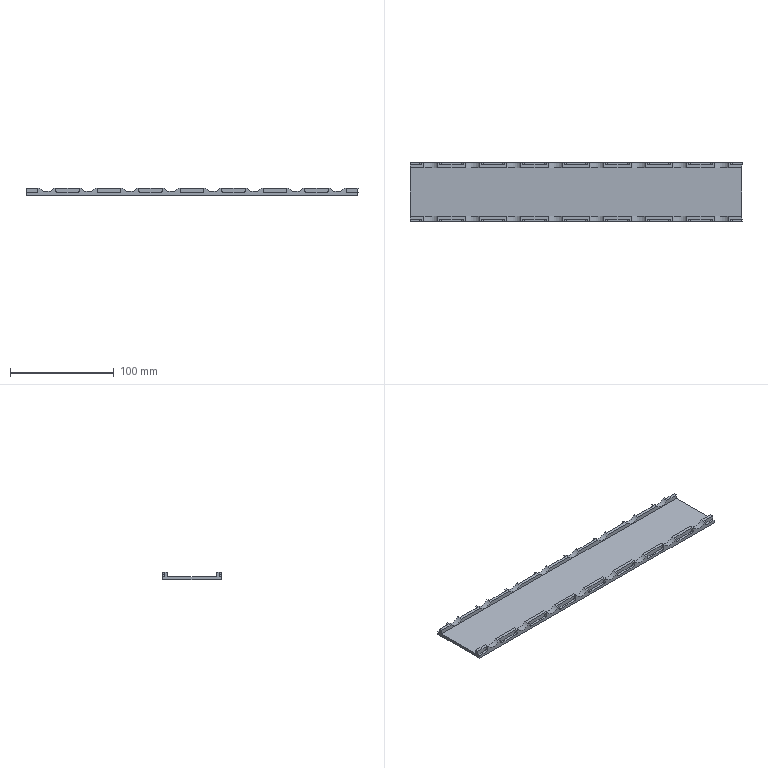NC program | Mastercam | posted with a generic post
Lines 1818 to 3883 of 9376, first 1896 of 2066 lines:
(8 FI |TOOL - 2|DIA. OFF. - 2|LEN. - 2|TOOL DIA. - 8.)
N3712 T2 M6
N3714 G0 G54 G90 X15.673 Y149.159 C0. B-90. S5000 M3
N3716 G43 H2 Z78.3
N3718 Z29.3
N3720 G1 Z22.3 F2000.
N3722 G41 D2 X9.609 Y143.942 F600.
N3724 G3 X7.8 Y140. I3.391 J-3.942
N3726 X9.609 Y136.058 I5.2
N3728 G1 G40 X15.673 Y130.841
N3730 G0 Z78.3
N3732 Y109.159
N3734 Z29.3
N3736 G1 Z22.3 F2000.
N3738 G41 D2 X9.609 Y103.942 F600.
N3740 G3 X7.8 Y100. I3.391 J-3.942
N3742 X9.609 Y96.058 I5.2
N3744 G1 G40 X15.673 Y90.841
N3746 G0 Z78.3
N3748 Y69.159
N3750 Z29.3
N3752 G1 Z22.3 F2000.
N3754 G41 D2 X9.609 Y63.942 F600.
N3756 G3 X7.8 Y60. I3.391 J-3.942
N3758 X9.609 Y56.058 I5.2
N3760 G1 G40 X15.673 Y50.841
N3762 G0 Z78.3
N3764 Y29.159
N3766 Z29.3
N3768 G1 Z22.3 F2000.
N3770 G41 D2 X9.609 Y23.942 F600.
N3772 G3 X7.8 Y20. I3.391 J-3.942
N3774 X9.609 Y16.058 I5.2
N3776 G1 G40 X15.673 Y10.841
N3778 G0 Z78.3
N3780 Y-10.841
N3782 Z29.3
N3784 G1 Z22.3 F2000.
N3786 G41 D2 X9.609 Y-16.058 F600.
N3788 G3 X7.8 Y-20. I3.391 J-3.942
N3790 X9.609 Y-23.942 I5.2
N3792 G1 G40 X15.673 Y-29.159
N3794 G0 Z78.3
N3796 Y-50.841
N3798 Z29.3
N3800 G1 Z22.3 F2000.
N3802 G41 D2 X9.609 Y-56.058 F600.
N3804 G3 X7.8 Y-60. I3.391 J-3.942
N3806 X9.609 Y-63.942 I5.2
N3808 G1 G40 X15.673 Y-69.159
N3810 G0 Z78.3
N3812 Y-90.841
N3814 Z29.3
N3816 G1 Z22.3 F2000.
N3818 G41 D2 X9.609 Y-96.058 F600.
N3820 G3 X7.8 Y-100. I3.391 J-3.942
N3822 X9.609 Y-103.942 I5.2
N3824 G1 G40 X15.673 Y-109.159
N3826 G0 Z78.3
N3828 Y-130.841
N3830 Z29.3
N3832 G1 Z22.3 F2000.
N3834 G41 D2 X9.609 Y-136.058 F600.
N3836 G3 X7.8 Y-140. I3.391 J-3.942
N3838 X9.609 Y-143.942 I5.2
N3840 G1 G40 X15.673 Y-149.159
N3842 G0 Z78.3
N3844 M5
N3846 G0 G28 G91 Z0.
N3848 G28 B0.
N3850 M01
N3852 G0 G17 G40 G80 G90 G94 G98
N3854 G0 G28 G91 Z0.
(4 RC |TOOL - 3|DIA. OFF. - 3|LEN. - 3|TOOL DIA. - 4.)
N3856 T3 M6
N3858 G0 G54 G90 X5.1 Y164. C0. B-90. S6500 M3
N3860 G43 H3 Z78.3
N3862 Z32.3
N3864 G1 Z31. F2000.
N3866 G41 D3 Y160. F600.
N3868 Y150.6
N3870 X7.
N3872 G40 X11.
N3874 Z30.7 F2000.
N3876 G42 D3 X7. F600.
N3878 X5.1
N3880 Y160.
N3882 G40 Y164.
N3884 Z30.4 F2000.
N3886 G41 D3 Y160. F600.
N3888 Y150.6
N3890 X7.
N3892 G40 X11.
N3894 Z30.1 F2000.
N3896 G42 D3 X7. F600.
N3898 X5.1
N3900 Y160.
N3902 G40 Y164.
N3904 Z29.8 F2000.
N3906 G41 D3 Y160. F600.
N3908 Y150.6
N3910 X7.
N3912 G40 X11.
N3914 Z29.5 F2000.
N3916 G42 D3 X7. F600.
N3918 X5.1
N3920 Y160.
N3922 G40 Y164.
N3924 Z29.2 F2000.
N3926 G41 D3 Y160. F600.
N3928 Y150.6
N3930 X7.
N3932 G40 X11.
N3934 Z28.9 F2000.
N3936 G42 D3 X7. F600.
N3938 X5.1
N3940 Y160.
N3942 G40 Y164.
N3944 Z28.6 F2000.
N3946 G41 D3 Y160. F600.
N3948 Y150.6
N3950 X7.
N3952 G40 X11.
N3954 Z28.3 F2000.
N3956 G42 D3 X7. F600.
N3958 X5.1
N3960 Y160.
N3962 G40 Y164.
N3964 Z28. F2000.
N3966 G41 D3 Y160. F600.
N3968 Y150.6
N3970 X7.
N3972 G40 X11.
N3974 Z27.7 F2000.
N3976 G42 D3 X7. F600.
N3978 X5.1
N3980 Y160.
N3982 G40 Y164.
N3984 Z27.4 F2000.
N3986 G41 D3 Y160. F600.
N3988 Y150.6
N3990 X7.
N3992 G40 X11.
N3994 Z27.1 F2000.
N3996 G42 D3 X7. F600.
N3998 X5.1
N4000 Y160.
N4002 G40 Y164.
N4004 Z26.8 F2000.
N4006 G41 D3 Y160. F600.
N4008 Y150.6
N4010 X7.
N4012 G40 X11.
N4014 Z26.5 F2000.
N4016 G42 D3 X7. F600.
N4018 X5.1
N4020 Y160.
N4022 G40 Y164.
N4024 Z26.2 F2000.
N4026 G41 D3 Y160. F600.
N4028 Y150.6
N4030 X7.
N4032 G40 X11.
N4034 G0 Z78.3
N4036 Y129.4
N4038 Z32.3
N4040 G1 Z31. F2000.
N4042 G41 D3 X7. F600.
N4044 X5.1
N4046 Y110.6
N4048 X7.
N4050 G40 X11.
N4052 Z30.7 F2000.
N4054 G42 D3 X7. F600.
N4056 X5.1
N4058 Y129.4
N4060 X7.
N4062 G40 X11.
N4064 Z30.4 F2000.
N4066 G41 D3 X7. F600.
N4068 X5.1
N4070 Y110.6
N4072 X7.
N4074 G40 X11.
N4076 Z30.1 F2000.
N4078 G42 D3 X7. F600.
N4080 X5.1
N4082 Y129.4
N4084 X7.
N4086 G40 X11.
N4088 Z29.8 F2000.
N4090 G41 D3 X7. F600.
N4092 X5.1
N4094 Y110.6
N4096 X7.
N4098 G40 X11.
N4100 Z29.5 F2000.
N4102 G42 D3 X7. F600.
N4104 X5.1
N4106 Y129.4
N4108 X7.
N4110 G40 X11.
N4112 Z29.2 F2000.
N4114 G41 D3 X7. F600.
N4116 X5.1
N4118 Y110.6
N4120 X7.
N4122 G40 X11.
N4124 Z28.9 F2000.
N4126 G42 D3 X7. F600.
N4128 X5.1
N4130 Y129.4
N4132 X7.
N4134 G40 X11.
N4136 Z28.6 F2000.
N4138 G41 D3 X7. F600.
N4140 X5.1
N4142 Y110.6
N4144 X7.
N4146 G40 X11.
N4148 Z28.3 F2000.
N4150 G42 D3 X7. F600.
N4152 X5.1
N4154 Y129.4
N4156 X7.
N4158 G40 X11.
N4160 Z28. F2000.
N4162 G41 D3 X7. F600.
N4164 X5.1
N4166 Y110.6
N4168 X7.
N4170 G40 X11.
N4172 Z27.7 F2000.
N4174 G42 D3 X7. F600.
N4176 X5.1
N4178 Y129.4
N4180 X7.
N4182 G40 X11.
N4184 Z27.4 F2000.
N4186 G41 D3 X7. F600.
N4188 X5.1
N4190 Y110.6
N4192 X7.
N4194 G40 X11.
N4196 Z27.1 F2000.
N4198 G42 D3 X7. F600.
N4200 X5.1
N4202 Y129.4
N4204 X7.
N4206 G40 X11.
N4208 Z26.8 F2000.
N4210 G41 D3 X7. F600.
N4212 X5.1
N4214 Y110.6
N4216 X7.
N4218 G40 X11.
N4220 Z26.5 F2000.
N4222 G42 D3 X7. F600.
N4224 X5.1
N4226 Y129.4
N4228 X7.
N4230 G40 X11.
N4232 Z26.2 F2000.
N4234 G41 D3 X7. F600.
N4236 X5.1
N4238 Y110.6
N4240 X7.
N4242 G40 X11.
N4244 G0 Z78.3
N4246 Y89.4
N4248 Z32.3
N4250 G1 Z31. F2000.
N4252 G41 D3 X7. F600.
N4254 X5.1
N4256 Y70.6
N4258 X7.
N4260 G40 X11.
N4262 Z30.7 F2000.
N4264 G42 D3 X7. F600.
N4266 X5.1
N4268 Y89.4
N4270 X7.
N4272 G40 X11.
N4274 Z30.4 F2000.
N4276 G41 D3 X7. F600.
N4278 X5.1
N4280 Y70.6
N4282 X7.
N4284 G40 X11.
N4286 Z30.1 F2000.
N4288 G42 D3 X7. F600.
N4290 X5.1
N4292 Y89.4
N4294 X7.
N4296 G40 X11.
N4298 Z29.8 F2000.
N4300 G41 D3 X7. F600.
N4302 X5.1
N4304 Y70.6
N4306 X7.
N4308 G40 X11.
N4310 Z29.5 F2000.
N4312 G42 D3 X7. F600.
N4314 X5.1
N4316 Y89.4
N4318 X7.
N4320 G40 X11.
N4322 Z29.2 F2000.
N4324 G41 D3 X7. F600.
N4326 X5.1
N4328 Y70.6
N4330 X7.
N4332 G40 X11.
N4334 Z28.9 F2000.
N4336 G42 D3 X7. F600.
N4338 X5.1
N4340 Y89.4
N4342 X7.
N4344 G40 X11.
N4346 Z28.6 F2000.
N4348 G41 D3 X7. F600.
N4350 X5.1
N4352 Y70.6
N4354 X7.
N4356 G40 X11.
N4358 Z28.3 F2000.
N4360 G42 D3 X7. F600.
N4362 X5.1
N4364 Y89.4
N4366 X7.
N4368 G40 X11.
N4370 Z28. F2000.
N4372 G41 D3 X7. F600.
N4374 X5.1
N4376 Y70.6
N4378 X7.
N4380 G40 X11.
N4382 Z27.7 F2000.
N4384 G42 D3 X7. F600.
N4386 X5.1
N4388 Y89.4
N4390 X7.
N4392 G40 X11.
N4394 Z27.4 F2000.
N4396 G41 D3 X7. F600.
N4398 X5.1
N4400 Y70.6
N4402 X7.
N4404 G40 X11.
N4406 Z27.1 F2000.
N4408 G42 D3 X7. F600.
N4410 X5.1
N4412 Y89.4
N4414 X7.
N4416 G40 X11.
N4418 Z26.8 F2000.
N4420 G41 D3 X7. F600.
N4422 X5.1
N4424 Y70.6
N4426 X7.
N4428 G40 X11.
N4430 Z26.5 F2000.
N4432 G42 D3 X7. F600.
N4434 X5.1
N4436 Y89.4
N4438 X7.
N4440 G40 X11.
N4442 Z26.2 F2000.
N4444 G41 D3 X7. F600.
N4446 X5.1
N4448 Y70.6
N4450 X7.
N4452 G40 X11.
N4454 G0 Z78.3
N4456 Y49.4
N4458 Z32.3
N4460 G1 Z31. F2000.
N4462 G41 D3 X7. F600.
N4464 X5.1
N4466 Y30.6
N4468 X7.
N4470 G40 X11.
N4472 Z30.7 F2000.
N4474 G42 D3 X7. F600.
N4476 X5.1
N4478 Y49.4
N4480 X7.
N4482 G40 X11.
N4484 Z30.4 F2000.
N4486 G41 D3 X7. F600.
N4488 X5.1
N4490 Y30.6
N4492 X7.
N4494 G40 X11.
N4496 Z30.1 F2000.
N4498 G42 D3 X7. F600.
N4500 X5.1
N4502 Y49.4
N4504 X7.
N4506 G40 X11.
N4508 Z29.8 F2000.
N4510 G41 D3 X7. F600.
N4512 X5.1
N4514 Y30.6
N4516 X7.
N4518 G40 X11.
N4520 Z29.5 F2000.
N4522 G42 D3 X7. F600.
N4524 X5.1
N4526 Y49.4
N4528 X7.
N4530 G40 X11.
N4532 Z29.2 F2000.
N4534 G41 D3 X7. F600.
N4536 X5.1
N4538 Y30.6
N4540 X7.
N4542 G40 X11.
N4544 Z28.9 F2000.
N4546 G42 D3 X7. F600.
N4548 X5.1
N4550 Y49.4
N4552 X7.
N4554 G40 X11.
N4556 Z28.6 F2000.
N4558 G41 D3 X7. F600.
N4560 X5.1
N4562 Y30.6
N4564 X7.
N4566 G40 X11.
N4568 Z28.3 F2000.
N4570 G42 D3 X7. F600.
N4572 X5.1
N4574 Y49.4
N4576 X7.
N4578 G40 X11.
N4580 Z28. F2000.
N4582 G41 D3 X7. F600.
N4584 X5.1
N4586 Y30.6
N4588 X7.
N4590 G40 X11.
N4592 Z27.7 F2000.
N4594 G42 D3 X7. F600.
N4596 X5.1
N4598 Y49.4
N4600 X7.
N4602 G40 X11.
N4604 Z27.4 F2000.
N4606 G41 D3 X7. F600.
N4608 X5.1
N4610 Y30.6
N4612 X7.
N4614 G40 X11.
N4616 Z27.1 F2000.
N4618 G42 D3 X7. F600.
N4620 X5.1
N4622 Y49.4
N4624 X7.
N4626 G40 X11.
N4628 Z26.8 F2000.
N4630 G41 D3 X7. F600.
N4632 X5.1
N4634 Y30.6
N4636 X7.
N4638 G40 X11.
N4640 Z26.5 F2000.
N4642 G42 D3 X7. F600.
N4644 X5.1
N4646 Y49.4
N4648 X7.
N4650 G40 X11.
N4652 Z26.2 F2000.
N4654 G41 D3 X7. F600.
N4656 X5.1
N4658 Y30.6
N4660 X7.
N4662 G40 X11.
N4664 G0 Z78.3
N4666 Y9.4
N4668 Z32.3
N4670 G1 Z31. F2000.
N4672 G41 D3 X7. F600.
N4674 X5.1
N4676 Y-9.4
N4678 X7.
N4680 G40 X11.
N4682 Z30.7 F2000.
N4684 G42 D3 X7. F600.
N4686 X5.1
N4688 Y9.4
N4690 X7.
N4692 G40 X11.
N4694 Z30.4 F2000.
N4696 G41 D3 X7. F600.
N4698 X5.1
N4700 Y-9.4
N4702 X7.
N4704 G40 X11.
N4706 Z30.1 F2000.
N4708 G42 D3 X7. F600.
N4710 X5.1
N4712 Y9.4
N4714 X7.
N4716 G40 X11.
N4718 Z29.8 F2000.
N4720 G41 D3 X7. F600.
N4722 X5.1
N4724 Y-9.4
N4726 X7.
N4728 G40 X11.
N4730 Z29.5 F2000.
N4732 G42 D3 X7. F600.
N4734 X5.1
N4736 Y9.4
N4738 X7.
N4740 G40 X11.
N4742 Z29.2 F2000.
N4744 G41 D3 X7. F600.
N4746 X5.1
N4748 Y-9.4
N4750 X7.
N4752 G40 X11.
N4754 Z28.9 F2000.
N4756 G42 D3 X7. F600.
N4758 X5.1
N4760 Y9.4
N4762 X7.
N4764 G40 X11.
N4766 Z28.6 F2000.
N4768 G41 D3 X7. F600.
N4770 X5.1
N4772 Y-9.4
N4774 X7.
N4776 G40 X11.
N4778 Z28.3 F2000.
N4780 G42 D3 X7. F600.
N4782 X5.1
N4784 Y9.4
N4786 X7.
N4788 G40 X11.
N4790 Z28. F2000.
N4792 G41 D3 X7. F600.
N4794 X5.1
N4796 Y-9.4
N4798 X7.
N4800 G40 X11.
N4802 Z27.7 F2000.
N4804 G42 D3 X7. F600.
N4806 X5.1
N4808 Y9.4
N4810 X7.
N4812 G40 X11.
N4814 Z27.4 F2000.
N4816 G41 D3 X7. F600.
N4818 X5.1
N4820 Y-9.4
N4822 X7.
N4824 G40 X11.
N4826 Z27.1 F2000.
N4828 G42 D3 X7. F600.
N4830 X5.1
N4832 Y9.4
N4834 X7.
N4836 G40 X11.
N4838 Z26.8 F2000.
N4840 G41 D3 X7. F600.
N4842 X5.1
N4844 Y-9.4
N4846 X7.
N4848 G40 X11.
N4850 Z26.5 F2000.
N4852 G42 D3 X7. F600.
N4854 X5.1
N4856 Y9.4
N4858 X7.
N4860 G40 X11.
N4862 Z26.2 F2000.
N4864 G41 D3 X7. F600.
N4866 X5.1
N4868 Y-9.4
N4870 X7.
N4872 G40 X11.
N4874 G0 Z78.3
N4876 Y-30.6
N4878 Z32.3
N4880 G1 Z31. F2000.
N4882 G41 D3 X7. F600.
N4884 X5.1
N4886 Y-49.4
N4888 X7.
N4890 G40 X11.
N4892 Z30.7 F2000.
N4894 G42 D3 X7. F600.
N4896 X5.1
N4898 Y-30.6
N4900 X7.
N4902 G40 X11.
N4904 Z30.4 F2000.
N4906 G41 D3 X7. F600.
N4908 X5.1
N4910 Y-49.4
N4912 X7.
N4914 G40 X11.
N4916 Z30.1 F2000.
N4918 G42 D3 X7. F600.
N4920 X5.1
N4922 Y-30.6
N4924 X7.
N4926 G40 X11.
N4928 Z29.8 F2000.
N4930 G41 D3 X7. F600.
N4932 X5.1
N4934 Y-49.4
N4936 X7.
N4938 G40 X11.
N4940 Z29.5 F2000.
N4942 G42 D3 X7. F600.
N4944 X5.1
N4946 Y-30.6
N4948 X7.
N4950 G40 X11.
N4952 Z29.2 F2000.
N4954 G41 D3 X7. F600.
N4956 X5.1
N4958 Y-49.4
N4960 X7.
N4962 G40 X11.
N4964 Z28.9 F2000.
N4966 G42 D3 X7. F600.
N4968 X5.1
N4970 Y-30.6
N4972 X7.
N4974 G40 X11.
N4976 Z28.6 F2000.
N4978 G41 D3 X7. F600.
N4980 X5.1
N4982 Y-49.4
N4984 X7.
N4986 G40 X11.
N4988 Z28.3 F2000.
N4990 G42 D3 X7. F600.
N4992 X5.1
N4994 Y-30.6
N4996 X7.
N4998 G40 X11.
N5000 Z28. F2000.
N5002 G41 D3 X7. F600.
N5004 X5.1
N5006 Y-49.4
N5008 X7.
N5010 G40 X11.
N5012 Z27.7 F2000.
N5014 G42 D3 X7. F600.
N5016 X5.1
N5018 Y-30.6
N5020 X7.
N5022 G40 X11.
N5024 Z27.4 F2000.
N5026 G41 D3 X7. F600.
N5028 X5.1
N5030 Y-49.4
N5032 X7.
N5034 G40 X11.
N5036 Z27.1 F2000.
N5038 G42 D3 X7. F600.
N5040 X5.1
N5042 Y-30.6
N5044 X7.
N5046 G40 X11.
N5048 Z26.8 F2000.
N5050 G41 D3 X7. F600.
N5052 X5.1
N5054 Y-49.4
N5056 X7.
N5058 G40 X11.
N5060 Z26.5 F2000.
N5062 G42 D3 X7. F600.
N5064 X5.1
N5066 Y-30.6
N5068 X7.
N5070 G40 X11.
N5072 Z26.2 F2000.
N5074 G41 D3 X7. F600.
N5076 X5.1
N5078 Y-49.4
N5080 X7.
N5082 G40 X11.
N5084 G0 Z78.3
N5086 Y-70.6
N5088 Z32.3
N5090 G1 Z31. F2000.
N5092 G41 D3 X7. F600.
N5094 X5.1
N5096 Y-89.4
N5098 X7.
N5100 G40 X11.
N5102 Z30.7 F2000.
N5104 G42 D3 X7. F600.
N5106 X5.1
N5108 Y-70.6
N5110 X7.
N5112 G40 X11.
N5114 Z30.4 F2000.
N5116 G41 D3 X7. F600.
N5118 X5.1
N5120 Y-89.4
N5122 X7.
N5124 G40 X11.
N5126 Z30.1 F2000.
N5128 G42 D3 X7. F600.
N5130 X5.1
N5132 Y-70.6
N5134 X7.
N5136 G40 X11.
N5138 Z29.8 F2000.
N5140 G41 D3 X7. F600.
N5142 X5.1
N5144 Y-89.4
N5146 X7.
N5148 G40 X11.
N5150 Z29.5 F2000.
N5152 G42 D3 X7. F600.
N5154 X5.1
N5156 Y-70.6
N5158 X7.
N5160 G40 X11.
N5162 Z29.2 F2000.
N5164 G41 D3 X7. F600.
N5166 X5.1
N5168 Y-89.4
N5170 X7.
N5172 G40 X11.
N5174 Z28.9 F2000.
N5176 G42 D3 X7. F600.
N5178 X5.1
N5180 Y-70.6
N5182 X7.
N5184 G40 X11.
N5186 Z28.6 F2000.
N5188 G41 D3 X7. F600.
N5190 X5.1
N5192 Y-89.4
N5194 X7.
N5196 G40 X11.
N5198 Z28.3 F2000.
N5200 G42 D3 X7. F600.
N5202 X5.1
N5204 Y-70.6
N5206 X7.
N5208 G40 X11.
N5210 Z28. F2000.
N5212 G41 D3 X7. F600.
N5214 X5.1
N5216 Y-89.4
N5218 X7.
N5220 G40 X11.
N5222 Z27.7 F2000.
N5224 G42 D3 X7. F600.
N5226 X5.1
N5228 Y-70.6
N5230 X7.
N5232 G40 X11.
N5234 Z27.4 F2000.
N5236 G41 D3 X7. F600.
N5238 X5.1
N5240 Y-89.4
N5242 X7.
N5244 G40 X11.
N5246 Z27.1 F2000.
N5248 G42 D3 X7. F600.
N5250 X5.1
N5252 Y-70.6
N5254 X7.
N5256 G40 X11.
N5258 Z26.8 F2000.
N5260 G41 D3 X7. F600.
N5262 X5.1
N5264 Y-89.4
N5266 X7.
N5268 G40 X11.
N5270 Z26.5 F2000.
N5272 G42 D3 X7. F600.
N5274 X5.1
N5276 Y-70.6
N5278 X7.
N5280 G40 X11.
N5282 Z26.2 F2000.
N5284 G41 D3 X7. F600.
N5286 X5.1
N5288 Y-89.4
N5290 X7.
N5292 G40 X11.
N5294 G0 Z78.3
N5296 Y-110.6
N5298 Z32.3
N5300 G1 Z31. F2000.
N5302 G41 D3 X7. F600.
N5304 X5.1
N5306 Y-129.4
N5308 X7.
N5310 G40 X11.
N5312 Z30.7 F2000.
N5314 G42 D3 X7. F600.
N5316 X5.1
N5318 Y-110.6
N5320 X7.
N5322 G40 X11.
N5324 Z30.4 F2000.
N5326 G41 D3 X7. F600.
N5328 X5.1
N5330 Y-129.4
N5332 X7.
N5334 G40 X11.
N5336 Z30.1 F2000.
N5338 G42 D3 X7. F600.
N5340 X5.1
N5342 Y-110.6
N5344 X7.
N5346 G40 X11.
N5348 Z29.8 F2000.
N5350 G41 D3 X7. F600.
N5352 X5.1
N5354 Y-129.4
N5356 X7.
N5358 G40 X11.
N5360 Z29.5 F2000.
N5362 G42 D3 X7. F600.
N5364 X5.1
N5366 Y-110.6
N5368 X7.
N5370 G40 X11.
N5372 Z29.2 F2000.
N5374 G41 D3 X7. F600.
N5376 X5.1
N5378 Y-129.4
N5380 X7.
N5382 G40 X11.
N5384 Z28.9 F2000.
N5386 G42 D3 X7. F600.
N5388 X5.1
N5390 Y-110.6
N5392 X7.
N5394 G40 X11.
N5396 Z28.6 F2000.
N5398 G41 D3 X7. F600.
N5400 X5.1
N5402 Y-129.4
N5404 X7.
N5406 G40 X11.
N5408 Z28.3 F2000.
N5410 G42 D3 X7. F600.
N5412 X5.1
N5414 Y-110.6
N5416 X7.
N5418 G40 X11.
N5420 Z28. F2000.
N5422 G41 D3 X7. F600.
N5424 X5.1
N5426 Y-129.4
N5428 X7.
N5430 G40 X11.
N5432 Z27.7 F2000.
N5434 G42 D3 X7. F600.
N5436 X5.1
N5438 Y-110.6
N5440 X7.
N5442 G40 X11.
N5444 Z27.4 F2000.
N5446 G41 D3 X7. F600.
N5448 X5.1
N5450 Y-129.4
N5452 X7.
N5454 G40 X11.
N5456 Z27.1 F2000.
N5458 G42 D3 X7. F600.
N5460 X5.1
N5462 Y-110.6
N5464 X7.
N5466 G40 X11.
N5468 Z26.8 F2000.
N5470 G41 D3 X7. F600.
N5472 X5.1
N5474 Y-129.4
N5476 X7.
N5478 G40 X11.
N5480 Z26.5 F2000.
N5482 G42 D3 X7. F600.
N5484 X5.1
N5486 Y-110.6
N5488 X7.
N5490 G40 X11.
N5492 Z26.2 F2000.
N5494 G41 D3 X7. F600.
N5496 X5.1
N5498 Y-129.4
N5500 X7.
N5502 G40 X11.
N5504 G0 Z78.3
N5506 Y-150.6
N5508 Z32.3
N5510 G1 Z31. F2000.
N5512 G41 D3 X7. F600.
N5514 X5.1
N5516 Y-160.
N5518 G40 Y-164.
N5520 Z30.7 F2000.
N5522 G42 D3 Y-160. F600.
N5524 Y-150.6
N5526 X7.
N5528 G40 X11.
N5530 Z30.4 F2000.
N5532 G41 D3 X7. F600.
N5534 X5.1
N5536 Y-160.
N5538 G40 Y-164.
N5540 Z30.1 F2000.
N5542 G42 D3 Y-160. F600.
N5544 Y-150.6
N5546 X7.
N5548 G40 X11.
N5550 Z29.8 F2000.
N5552 G41 D3 X7. F600.
N5554 X5.1
N5556 Y-160.
N5558 G40 Y-164.
N5560 Z29.5 F2000.
N5562 G42 D3 Y-160. F600.
N5564 Y-150.6
N5566 X7.
N5568 G40 X11.
N5570 Z29.2 F2000.
N5572 G41 D3 X7. F600.
N5574 X5.1
N5576 Y-160.
N5578 G40 Y-164.
N5580 Z28.9 F2000.
N5582 G42 D3 Y-160. F600.
N5584 Y-150.6
N5586 X7.
N5588 G40 X11.
N5590 Z28.6 F2000.
N5592 G41 D3 X7. F600.
N5594 X5.1
N5596 Y-160.
N5598 G40 Y-164.
N5600 Z28.3 F2000.
N5602 G42 D3 Y-160. F600.
N5604 Y-150.6
N5606 X7.
N5608 G40 X11.
N5610 Z28. F2000.
N5612 G41 D3 X7. F600.
N5614 X5.1
N5616 Y-160.
N5618 G40 Y-164.
N5620 Z27.7 F2000.
N5622 G42 D3 Y-160. F600.
N5624 Y-150.6
N5626 X7.
N5628 G40 X11.
N5630 Z27.4 F2000.
N5632 G41 D3 X7. F600.
N5634 X5.1
N5636 Y-160.
N5638 G40 Y-164.
N5640 Z27.1 F2000.
N5642 G42 D3 Y-160. F600.
N5644 Y-150.6
N5646 X7.
N5648 G40 X11.
N5650 Z26.8 F2000.
N5652 G41 D3 X7. F600.
N5654 X5.1
N5656 Y-160.
N5658 G40 Y-164.
N5660 Z26.5 F2000.
N5662 G42 D3 Y-160. F600.
N5664 Y-150.6
N5666 X7.
N5668 G40 X11.
N5670 Z26.2 F2000.
N5672 G41 D3 X7. F600.
N5674 X5.1
N5676 Y-160.
N5678 G40 Y-164.
N5680 G0 Z78.3
N5682 M5
N5684 G0 G28 G91 Z0.
N5686 G28 B0.
N5688 M01
N5690 G0 G17 G40 G80 G90 G94 G98
N5692 G0 G28 G91 Z0.
(4 FI |TOOL - 4|DIA. OFF. - 4|LEN. - 4|TOOL DIA. - 4.)
N5694 T4 M6
N5696 G0 G54 G90 X6. Y164. C0. B-90. S6500 M3
N5698 G43 H4 Z78.3
N5700 Z32.3
N5702 G1 Z26.1 F2000.
N5704 G41 D4 Y160. F600.
N5706 Y151.5
N5708 X7.
N5710 G40 X11.
N5712 G0 Z78.3
N5714 X5. Y164.
N5716 Z32.3
N5718 G1 Z26.1 F2000.
N5720 G41 D4 Y160. F600.
N5722 Y150.5
N5724 X7.
N5726 G40 X11.
N5728 G0 Z78.3
N5730 Y128.5
N5732 Z32.3
N5734 G1 Z26.1 F2000.
N5736 G41 D4 X7. F600.
N5738 X6.
N5740 Y111.5
N5742 X7.
N5744 G40 X11.
N5746 G0 Z78.3
N5748 Y129.5
N5750 Z32.3
N5752 G1 Z26.1 F2000.
N5754 G41 D4 X7. F600.
N5756 X5.
N5758 Y110.5
N5760 X7.
N5762 G40 X11.
N5764 G0 Z78.3
N5766 Y88.5
N5768 Z32.3
N5770 G1 Z26.1 F2000.
N5772 G41 D4 X7. F600.
N5774 X6.
N5776 Y71.5
N5778 X7.
N5780 G40 X11.
N5782 G0 Z78.3
N5784 Y89.5
N5786 Z32.3
N5788 G1 Z26.1 F2000.
N5790 G41 D4 X7. F600.
N5792 X5.
N5794 Y70.5
N5796 X7.
N5798 G40 X11.
N5800 G0 Z78.3
N5802 Y48.5
N5804 Z32.3
N5806 G1 Z26.1 F2000.
N5808 G41 D4 X7. F600.
N5810 X6.
N5812 Y31.5
N5814 X7.
N5816 G40 X11.
N5818 G0 Z78.3
N5820 Y49.5
N5822 Z32.3
N5824 G1 Z26.1 F2000.
N5826 G41 D4 X7. F600.
N5828 X5.
N5830 Y30.5
N5832 X7.
N5834 G40 X11.
N5836 G0 Z78.3
N5838 Y8.5
N5840 Z32.3
N5842 G1 Z26.1 F2000.
N5844 G41 D4 X7. F600.
N5846 X6.
N5848 Y-8.5
N5850 X7.
N5852 G40 X11.
N5854 G0 Z78.3
N5856 Y9.5
N5858 Z32.3
N5860 G1 Z26.1 F2000.
N5862 G41 D4 X7. F600.
N5864 X5.
N5866 Y-9.5
N5868 X7.
N5870 G40 X11.
N5872 G0 Z78.3
N5874 Y-31.5
N5876 Z32.3
N5878 G1 Z26.1 F2000.
N5880 G41 D4 X7. F600.
N5882 X6.
N5884 Y-48.5
N5886 X7.
N5888 G40 X11.
N5890 G0 Z78.3
N5892 Y-30.5
N5894 Z32.3
N5896 G1 Z26.1 F2000.
N5898 G41 D4 X7. F600.
N5900 X5.
N5902 Y-49.5
N5904 X7.
N5906 G40 X11.
N5908 G0 Z78.3
N5910 Y-71.5
N5912 Z32.3
N5914 G1 Z26.1 F2000.
N5916 G41 D4 X7. F600.
N5918 X6.
N5920 Y-88.5
N5922 X7.
N5924 G40 X11.
N5926 G0 Z78.3
N5928 Y-70.5
N5930 Z32.3
N5932 G1 Z26.1 F2000.
N5934 G41 D4 X7. F600.
N5936 X5.
N5938 Y-89.5
N5940 X7.
N5942 G40 X11.
N5944 G0 Z78.3
N5946 Y-111.5
N5948 Z32.3
N5950 G1 Z26.1 F2000.
N5952 G41 D4 X7. F600.
N5954 X6.
N5956 Y-128.5
N5958 X7.
N5960 G40 X11.
N5962 G0 Z78.3
N5964 Y-110.5
N5966 Z32.3
N5968 G1 Z26.1 F2000.
N5970 G41 D4 X7. F600.
N5972 X5.
N5974 Y-129.5
N5976 X7.
N5978 G40 X11.
N5980 G0 Z78.3
N5982 Y-151.5
N5984 Z32.3
N5986 G1 Z26.1 F2000.
N5988 G41 D4 X7. F600.
N5990 X6.
N5992 Y-160.
N5994 G40 Y-164.
N5996 G0 Z78.3
N5998 X11. Y-150.5
N6000 Z32.3
N6002 G1 Z26.1 F2000.
N6004 G41 D4 X7. F600.
N6006 X5.
N6008 Y-160.
N6010 G40 Y-164.
N6012 G0 Z78.3
N6014 M5
N6016 G0 G28 G91 Z0.
N6018 G28 B0.
N6020 M01
N6022 G0 G17 G40 G80 G90 G94 G98
N6024 G0 G28 G91 Z0.
(8  RC |TOOL - 1|DIA. OFF. - 1|LEN. - 1|TOOL DIA. - 8.)
N6026 T1 M6
N6028 G0 G54 G90 X15.771 Y-130.954 C180. B-90. S5000 M3
N6030 G43 H1 Z78.3
N6032 Z33.3
N6034 G1 Z31.8 F2000.
N6036 G41 D1 X9.707 Y-136.172 F1000.
N6038 G3 X7.951 Y-140. I3.293 J-3.828
N6040 X9.707 Y-143.828 I5.049
N6042 G1 G40 X15.771 Y-149.046
N6044 Z31.3 F2000.
N6046 G42 D1 X9.707 Y-143.828 F1000.
N6048 G2 X7.951 Y-140. I3.293 J3.828
N6050 X9.707 Y-136.172 I5.049
N6052 G1 G40 X15.771 Y-130.954
N6054 Z30.8 F2000.
N6056 G41 D1 X9.707 Y-136.172 F1000.
N6058 G3 X7.951 Y-140. I3.293 J-3.828
N6060 X9.707 Y-143.828 I5.049
N6062 G1 G40 X15.771 Y-149.046
N6064 Z30.3 F2000.
N6066 G42 D1 X9.707 Y-143.828 F1000.
N6068 G2 X7.951 Y-140. I3.293 J3.828
N6070 X9.707 Y-136.172 I5.049
N6072 G1 G40 X15.771 Y-130.954
N6074 Z29.8 F2000.
N6076 G41 D1 X9.707 Y-136.172 F1000.
N6078 G3 X7.951 Y-140. I3.293 J-3.828
N6080 X9.707 Y-143.828 I5.049
N6082 G1 G40 X15.771 Y-149.046
N6084 Z29.3 F2000.
N6086 G42 D1 X9.707 Y-143.828 F1000.
N6088 G2 X7.951 Y-140. I3.293 J3.828
N6090 X9.707 Y-136.172 I5.049
N6092 G1 G40 X15.771 Y-130.954
N6094 Z28.8 F2000.
N6096 G41 D1 X9.707 Y-136.172 F1000.
N6098 G3 X7.951 Y-140. I3.293 J-3.828
N6100 X9.707 Y-143.828 I5.049
N6102 G1 G40 X15.771 Y-149.046
N6104 Z28.3 F2000.
N6106 G42 D1 X9.707 Y-143.828 F1000.
N6108 G2 X7.951 Y-140. I3.293 J3.828
N6110 X9.707 Y-136.172 I5.049
N6112 G1 G40 X15.771 Y-130.954
N6114 Z27.8 F2000.
N6116 G41 D1 X9.707 Y-136.172 F1000.
N6118 G3 X7.951 Y-140. I3.293 J-3.828
N6120 X9.707 Y-143.828 I5.049
N6122 G1 G40 X15.771 Y-149.046
N6124 Z27.3 F2000.
N6126 G42 D1 X9.707 Y-143.828 F1000.
N6128 G2 X7.951 Y-140. I3.293 J3.828
N6130 X9.707 Y-136.172 I5.049
N6132 G1 G40 X15.771 Y-130.954
N6134 Z26.8 F2000.
N6136 G41 D1 X9.707 Y-136.172 F1000.
N6138 G3 X7.951 Y-140. I3.293 J-3.828
N6140 X9.707 Y-143.828 I5.049
N6142 G1 G40 X15.771 Y-149.046
N6144 Z26.3 F2000.
N6146 G42 D1 X9.707 Y-143.828 F1000.
N6148 G2 X7.951 Y-140. I3.293 J3.828
N6150 X9.707 Y-136.172 I5.049
N6152 G1 G40 X15.771 Y-130.954
N6154 Z25.8 F2000.
N6156 G41 D1 X9.707 Y-136.172 F1000.
N6158 G3 X7.951 Y-140. I3.293 J-3.828
N6160 X9.707 Y-143.828 I5.049
N6162 G1 G40 X15.771 Y-149.046
N6164 Z25.3 F2000.
N6166 G42 D1 X9.707 Y-143.828 F1000.
N6168 G2 X7.951 Y-140. I3.293 J3.828
N6170 X9.707 Y-136.172 I5.049
N6172 G1 G40 X15.771 Y-130.954
N6174 Z24.8 F2000.
N6176 G41 D1 X9.707 Y-136.172 F1000.
N6178 G3 X7.951 Y-140. I3.293 J-3.828
N6180 X9.707 Y-143.828 I5.049
N6182 G1 G40 X15.771 Y-149.046
N6184 Z24.3 F2000.
N6186 G42 D1 X9.707 Y-143.828 F1000.
N6188 G2 X7.951 Y-140. I3.293 J3.828
N6190 X9.707 Y-136.172 I5.049
N6192 G1 G40 X15.771 Y-130.954
N6194 Z23.8 F2000.
N6196 G41 D1 X9.707 Y-136.172 F1000.
N6198 G3 X7.951 Y-140. I3.293 J-3.828
N6200 X9.707 Y-143.828 I5.049
N6202 G1 G40 X15.771 Y-149.046
N6204 Z23.3 F2000.
N6206 G42 D1 X9.707 Y-143.828 F1000.
N6208 G2 X7.951 Y-140. I3.293 J3.828
N6210 X9.707 Y-136.172 I5.049
N6212 G1 G40 X15.771 Y-130.954
N6214 Z22.8 F2000.
N6216 G41 D1 X9.707 Y-136.172 F1000.
N6218 G3 X7.951 Y-140. I3.293 J-3.828
N6220 X9.707 Y-143.828 I5.049
N6222 G1 G40 X15.771 Y-149.046
N6224 Z22.3 F2000.
N6226 G42 D1 X9.707 Y-143.828 F1000.
N6228 G2 X7.951 Y-140. I3.293 J3.828
N6230 X9.707 Y-136.172 I5.049
N6232 G1 G40 X15.771 Y-130.954
N6234 G0 Z78.3
N6236 Y-90.954
N6238 Z33.3
N6240 G1 Z31.8 F2000.
N6242 G41 D1 X9.707 Y-96.172 F1000.
N6244 G3 X7.951 Y-100. I3.293 J-3.828
N6246 X9.707 Y-103.828 I5.049
N6248 G1 G40 X15.771 Y-109.046
N6250 Z31.3 F2000.
N6252 G42 D1 X9.707 Y-103.828 F1000.
N6254 G2 X7.951 Y-100. I3.293 J3.828
N6256 X9.707 Y-96.172 I5.049
N6258 G1 G40 X15.771 Y-90.954
N6260 Z30.8 F2000.
N6262 G41 D1 X9.707 Y-96.172 F1000.
N6264 G3 X7.951 Y-100. I3.293 J-3.828
N6266 X9.707 Y-103.828 I5.049
N6268 G1 G40 X15.771 Y-109.046
N6270 Z30.3 F2000.
N6272 G42 D1 X9.707 Y-103.828 F1000.
N6274 G2 X7.951 Y-100. I3.293 J3.828
N6276 X9.707 Y-96.172 I5.049
N6278 G1 G40 X15.771 Y-90.954
N6280 Z29.8 F2000.
N6282 G41 D1 X9.707 Y-96.172 F1000.
N6284 G3 X7.951 Y-100. I3.293 J-3.828
N6286 X9.707 Y-103.828 I5.049
N6288 G1 G40 X15.771 Y-109.046
N6290 Z29.3 F2000.
N6292 G42 D1 X9.707 Y-103.828 F1000.
N6294 G2 X7.951 Y-100. I3.293 J3.828
N6296 X9.707 Y-96.172 I5.049
N6298 G1 G40 X15.771 Y-90.954
N6300 Z28.8 F2000.
N6302 G41 D1 X9.707 Y-96.172 F1000.
N6304 G3 X7.951 Y-100. I3.293 J-3.828
N6306 X9.707 Y-103.828 I5.049
N6308 G1 G40 X15.771 Y-109.046
N6310 Z28.3 F2000.
N6312 G42 D1 X9.707 Y-103.828 F1000.
N6314 G2 X7.951 Y-100. I3.293 J3.828
N6316 X9.707 Y-96.172 I5.049
N6318 G1 G40 X15.771 Y-90.954
N6320 Z27.8 F2000.
N6322 G41 D1 X9.707 Y-96.172 F1000.
N6324 G3 X7.951 Y-100. I3.293 J-3.828
N6326 X9.707 Y-103.828 I5.049
N6328 G1 G40 X15.771 Y-109.046
N6330 Z27.3 F2000.
N6332 G42 D1 X9.707 Y-103.828 F1000.
N6334 G2 X7.951 Y-100. I3.293 J3.828
N6336 X9.707 Y-96.172 I5.049
N6338 G1 G40 X15.771 Y-90.954
N6340 Z26.8 F2000.
N6342 G41 D1 X9.707 Y-96.172 F1000.
N6344 G3 X7.951 Y-100. I3.293 J-3.828
N6346 X9.707 Y-103.828 I5.049
N6348 G1 G40 X15.771 Y-109.046
N6350 Z26.3 F2000.
N6352 G42 D1 X9.707 Y-103.828 F1000.
N6354 G2 X7.951 Y-100. I3.293 J3.828
N6356 X9.707 Y-96.172 I5.049
N6358 G1 G40 X15.771 Y-90.954
N6360 Z25.8 F2000.
N6362 G41 D1 X9.707 Y-96.172 F1000.
N6364 G3 X7.951 Y-100. I3.293 J-3.828
N6366 X9.707 Y-103.828 I5.049
N6368 G1 G40 X15.771 Y-109.046
N6370 Z25.3 F2000.
N6372 G42 D1 X9.707 Y-103.828 F1000.
N6374 G2 X7.951 Y-100. I3.293 J3.828
N6376 X9.707 Y-96.172 I5.049
N6378 G1 G40 X15.771 Y-90.954
N6380 Z24.8 F2000.
N6382 G41 D1 X9.707 Y-96.172 F1000.
N6384 G3 X7.951 Y-100. I3.293 J-3.828
N6386 X9.707 Y-103.828 I5.049
N6388 G1 G40 X15.771 Y-109.046
N6390 Z24.3 F2000.
N6392 G42 D1 X9.707 Y-103.828 F1000.
N6394 G2 X7.951 Y-100. I3.293 J3.828
N6396 X9.707 Y-96.172 I5.049
N6398 G1 G40 X15.771 Y-90.954
N6400 Z23.8 F2000.
N6402 G41 D1 X9.707 Y-96.172 F1000.
N6404 G3 X7.951 Y-100. I3.293 J-3.828
N6406 X9.707 Y-103.828 I5.049
N6408 G1 G40 X15.771 Y-109.046
N6410 Z23.3 F2000.
N6412 G42 D1 X9.707 Y-103.828 F1000.
N6414 G2 X7.951 Y-100. I3.293 J3.828
N6416 X9.707 Y-96.172 I5.049
N6418 G1 G40 X15.771 Y-90.954
N6420 Z22.8 F2000.
N6422 G41 D1 X9.707 Y-96.172 F1000.
N6424 G3 X7.951 Y-100. I3.293 J-3.828
N6426 X9.707 Y-103.828 I5.049
N6428 G1 G40 X15.771 Y-109.046
N6430 Z22.3 F2000.
N6432 G42 D1 X9.707 Y-103.828 F1000.
N6434 G2 X7.951 Y-100. I3.293 J3.828
N6436 X9.707 Y-96.172 I5.049
N6438 G1 G40 X15.771 Y-90.954
N6440 G0 Z78.3
N6442 Y-50.954
N6444 Z33.3
N6446 G1 Z31.8 F2000.
N6448 G41 D1 X9.707 Y-56.172 F1000.
N6450 G3 X7.951 Y-60. I3.293 J-3.828
N6452 X9.707 Y-63.828 I5.049
N6454 G1 G40 X15.771 Y-69.046
N6456 Z31.3 F2000.
N6458 G42 D1 X9.707 Y-63.828 F1000.
N6460 G2 X7.951 Y-60. I3.293 J3.828
N6462 X9.707 Y-56.172 I5.049
N6464 G1 G40 X15.771 Y-50.954
N6466 Z30.8 F2000.
N6468 G41 D1 X9.707 Y-56.172 F1000.
N6470 G3 X7.951 Y-60. I3.293 J-3.828
N6472 X9.707 Y-63.828 I5.049
N6474 G1 G40 X15.771 Y-69.046
N6476 Z30.3 F2000.
N6478 G42 D1 X9.707 Y-63.828 F1000.
N6480 G2 X7.951 Y-60. I3.293 J3.828
N6482 X9.707 Y-56.172 I5.049
N6484 G1 G40 X15.771 Y-50.954
N6486 Z29.8 F2000.
N6488 G41 D1 X9.707 Y-56.172 F1000.
N6490 G3 X7.951 Y-60. I3.293 J-3.828
N6492 X9.707 Y-63.828 I5.049
N6494 G1 G40 X15.771 Y-69.046
N6496 Z29.3 F2000.
N6498 G42 D1 X9.707 Y-63.828 F1000.
N6500 G2 X7.951 Y-60. I3.293 J3.828
N6502 X9.707 Y-56.172 I5.049
N6504 G1 G40 X15.771 Y-50.954
N6506 Z28.8 F2000.
N6508 G41 D1 X9.707 Y-56.172 F1000.
N6510 G3 X7.951 Y-60. I3.293 J-3.828
N6512 X9.707 Y-63.828 I5.049
N6514 G1 G40 X15.771 Y-69.046
N6516 Z28.3 F2000.
N6518 G42 D1 X9.707 Y-63.828 F1000.
N6520 G2 X7.951 Y-60. I3.293 J3.828
N6522 X9.707 Y-56.172 I5.049
N6524 G1 G40 X15.771 Y-50.954
N6526 Z27.8 F2000.
N6528 G41 D1 X9.707 Y-56.172 F1000.
N6530 G3 X7.951 Y-60. I3.293 J-3.828
N6532 X9.707 Y-63.828 I5.049
N6534 G1 G40 X15.771 Y-69.046
N6536 Z27.3 F2000.
N6538 G42 D1 X9.707 Y-63.828 F1000.
N6540 G2 X7.951 Y-60. I3.293 J3.828
N6542 X9.707 Y-56.172 I5.049
N6544 G1 G40 X15.771 Y-50.954
N6546 Z26.8 F2000.
N6548 G41 D1 X9.707 Y-56.172 F1000.
N6550 G3 X7.951 Y-60. I3.293 J-3.828
N6552 X9.707 Y-63.828 I5.049
N6554 G1 G40 X15.771 Y-69.046
N6556 Z26.3 F2000.
N6558 G42 D1 X9.707 Y-63.828 F1000.
N6560 G2 X7.951 Y-60. I3.293 J3.828
N6562 X9.707 Y-56.172 I5.049
N6564 G1 G40 X15.771 Y-50.954
N6566 Z25.8 F2000.
N6568 G41 D1 X9.707 Y-56.172 F1000.
N6570 G3 X7.951 Y-60. I3.293 J-3.828
N6572 X9.707 Y-63.828 I5.049
N6574 G1 G40 X15.771 Y-69.046
N6576 Z25.3 F2000.
N6578 G42 D1 X9.707 Y-63.828 F1000.
N6580 G2 X7.951 Y-60. I3.293 J3.828
N6582 X9.707 Y-56.172 I5.049
N6584 G1 G40 X15.771 Y-50.954
N6586 Z24.8 F2000.
N6588 G41 D1 X9.707 Y-56.172 F1000.
N6590 G3 X7.951 Y-60. I3.293 J-3.828
N6592 X9.707 Y-63.828 I5.049
N6594 G1 G40 X15.771 Y-69.046
N6596 Z24.3 F2000.
N6598 G42 D1 X9.707 Y-63.828 F1000.
N6600 G2 X7.951 Y-60. I3.293 J3.828
N6602 X9.707 Y-56.172 I5.049
N6604 G1 G40 X15.771 Y-50.954
N6606 Z23.8 F2000.
N6608 G41 D1 X9.707 Y-56.172 F1000.
N6610 G3 X7.951 Y-60. I3.293 J-3.828
N6612 X9.707 Y-63.828 I5.049
N6614 G1 G40 X15.771 Y-69.046
N6616 Z23.3 F2000.
N6618 G42 D1 X9.707 Y-63.828 F1000.
N6620 G2 X7.951 Y-60. I3.293 J3.828
N6622 X9.707 Y-56.172 I5.049
N6624 G1 G40 X15.771 Y-50.954
N6626 Z22.8 F2000.
N6628 G41 D1 X9.707 Y-56.172 F1000.
N6630 G3 X7.951 Y-60. I3.293 J-3.828
N6632 X9.707 Y-63.828 I5.049
N6634 G1 G40 X15.771 Y-69.046
N6636 Z22.3 F2000.
N6638 G42 D1 X9.707 Y-63.828 F1000.
N6640 G2 X7.951 Y-60. I3.293 J3.828
N6642 X9.707 Y-56.172 I5.049
N6644 G1 G40 X15.771 Y-50.954
N6646 G0 Z78.3
N6648 Y-10.954
N6650 Z33.3
N6652 G1 Z31.8 F2000.
N6654 G41 D1 X9.707 Y-16.172 F1000.
N6656 G3 X7.951 Y-20. I3.293 J-3.828
N6658 X9.707 Y-23.828 I5.049
N6660 G1 G40 X15.771 Y-29.046
N6662 Z31.3 F2000.
N6664 G42 D1 X9.707 Y-23.828 F1000.
N6666 G2 X7.951 Y-20. I3.293 J3.828
N6668 X9.707 Y-16.172 I5.049
N6670 G1 G40 X15.771 Y-10.954
N6672 Z30.8 F2000.
N6674 G41 D1 X9.707 Y-16.172 F1000.
N6676 G3 X7.951 Y-20. I3.293 J-3.828
N6678 X9.707 Y-23.828 I5.049
N6680 G1 G40 X15.771 Y-29.046
N6682 Z30.3 F2000.
N6684 G42 D1 X9.707 Y-23.828 F1000.
N6686 G2 X7.951 Y-20. I3.293 J3.828
N6688 X9.707 Y-16.172 I5.049
N6690 G1 G40 X15.771 Y-10.954
N6692 Z29.8 F2000.
N6694 G41 D1 X9.707 Y-16.172 F1000.
N6696 G3 X7.951 Y-20. I3.293 J-3.828
N6698 X9.707 Y-23.828 I5.049
N6700 G1 G40 X15.771 Y-29.046
N6702 Z29.3 F2000.
N6704 G42 D1 X9.707 Y-23.828 F1000.
N6706 G2 X7.951 Y-20. I3.293 J3.828
N6708 X9.707 Y-16.172 I5.049
N6710 G1 G40 X15.771 Y-10.954
N6712 Z28.8 F2000.
N6714 G41 D1 X9.707 Y-16.172 F1000.
N6716 G3 X7.951 Y-20. I3.293 J-3.828
N6718 X9.707 Y-23.828 I5.049
N6720 G1 G40 X15.771 Y-29.046
N6722 Z28.3 F2000.
N6724 G42 D1 X9.707 Y-23.828 F1000.
N6726 G2 X7.951 Y-20. I3.293 J3.828
N6728 X9.707 Y-16.172 I5.049
N6730 G1 G40 X15.771 Y-10.954
N6732 Z27.8 F2000.
N6734 G41 D1 X9.707 Y-16.172 F1000.
N6736 G3 X7.951 Y-20. I3.293 J-3.828
N6738 X9.707 Y-23.828 I5.049
N6740 G1 G40 X15.771 Y-29.046
N6742 Z27.3 F2000.
N6744 G42 D1 X9.707 Y-23.828 F1000.
N6746 G2 X7.951 Y-20. I3.293 J3.828
N6748 X9.707 Y-16.172 I5.049
N6750 G1 G40 X15.771 Y-10.954
N6752 Z26.8 F2000.
N6754 G41 D1 X9.707 Y-16.172 F1000.
N6756 G3 X7.951 Y-20. I3.293 J-3.828
N6758 X9.707 Y-23.828 I5.049
N6760 G1 G40 X15.771 Y-29.046
N6762 Z26.3 F2000.
N6764 G42 D1 X9.707 Y-23.828 F1000.
N6766 G2 X7.951 Y-20. I3.293 J3.828
N6768 X9.707 Y-16.172 I5.049
N6770 G1 G40 X15.771 Y-10.954
N6772 Z25.8 F2000.
N6774 G41 D1 X9.707 Y-16.172 F1000.
N6776 G3 X7.951 Y-20. I3.293 J-3.828
N6778 X9.707 Y-23.828 I5.049
N6780 G1 G40 X15.771 Y-29.046
N6782 Z25.3 F2000.
N6784 G42 D1 X9.707 Y-23.828 F1000.
N6786 G2 X7.951 Y-20. I3.293 J3.828
N6788 X9.707 Y-16.172 I5.049
N6790 G1 G40 X15.771 Y-10.954
N6792 Z24.8 F2000.
N6794 G41 D1 X9.707 Y-16.172 F1000.
N6796 G3 X7.951 Y-20. I3.293 J-3.828
N6798 X9.707 Y-23.828 I5.049
N6800 G1 G40 X15.771 Y-29.046
N6802 Z24.3 F2000.
N6804 G42 D1 X9.707 Y-23.828 F1000.
N6806 G2 X7.951 Y-20. I3.293 J3.828
N6808 X9.707 Y-16.172 I5.049
N6810 G1 G40 X15.771 Y-10.954
N6812 Z23.8 F2000.
N6814 G41 D1 X9.707 Y-16.172 F1000.
N6816 G3 X7.951 Y-20. I3.293 J-3.828
N6818 X9.707 Y-23.828 I5.049
N6820 G1 G40 X15.771 Y-29.046
N6822 Z23.3 F2000.
N6824 G42 D1 X9.707 Y-23.828 F1000.
N6826 G2 X7.951 Y-20. I3.293 J3.828
N6828 X9.707 Y-16.172 I5.049
N6830 G1 G40 X15.771 Y-10.954
N6832 Z22.8 F2000.
N6834 G41 D1 X9.707 Y-16.172 F1000.
N6836 G3 X7.951 Y-20. I3.293 J-3.828
N6838 X9.707 Y-23.828 I5.049
N6840 G1 G40 X15.771 Y-29.046
N6842 Z22.3 F2000.
N6844 G42 D1 X9.707 Y-23.828 F1000.
N6846 G2 X7.951 Y-20. I3.293 J3.828
N6848 X9.707 Y-16.172 I5.049
N6850 G1 G40 X15.771 Y-10.954
N6852 G0 Z78.3
N6854 Y29.046
N6856 Z33.3
N6858 G1 Z31.8 F2000.
N6860 G41 D1 X9.707 Y23.828 F1000.
N6862 G3 X7.951 Y20. I3.293 J-3.828
N6864 X9.707 Y16.172 I5.049
N6866 G1 G40 X15.771 Y10.954
N6868 Z31.3 F2000.
N6870 G42 D1 X9.707 Y16.172 F1000.
N6872 G2 X7.951 Y20. I3.293 J3.828
N6874 X9.707 Y23.828 I5.049
N6876 G1 G40 X15.771 Y29.046
N6878 Z30.8 F2000.
N6880 G41 D1 X9.707 Y23.828 F1000.
N6882 G3 X7.951 Y20. I3.293 J-3.828
N6884 X9.707 Y16.172 I5.049
N6886 G1 G40 X15.771 Y10.954
N6888 Z30.3 F2000.
N6890 G42 D1 X9.707 Y16.172 F1000.
N6892 G2 X7.951 Y20. I3.293 J3.828
N6894 X9.707 Y23.828 I5.049
N6896 G1 G40 X15.771 Y29.046
N6898 Z29.8 F2000.
N6900 G41 D1 X9.707 Y23.828 F1000.
N6902 G3 X7.951 Y20. I3.293 J-3.828
N6904 X9.707 Y16.172 I5.049
N6906 G1 G40 X15.771 Y10.954
N6908 Z29.3 F2000.
N6910 G42 D1 X9.707 Y16.172 F1000.
N6912 G2 X7.951 Y20. I3.293 J3.828
N6914 X9.707 Y23.828 I5.049
N6916 G1 G40 X15.771 Y29.046
N6918 Z28.8 F2000.
N6920 G41 D1 X9.707 Y23.828 F1000.
N6922 G3 X7.951 Y20. I3.293 J-3.828
N6924 X9.707 Y16.172 I5.049
N6926 G1 G40 X15.771 Y10.954
N6928 Z28.3 F2000.
N6930 G42 D1 X9.707 Y16.172 F1000.
N6932 G2 X7.951 Y20. I3.293 J3.828
N6934 X9.707 Y23.828 I5.049
N6936 G1 G40 X15.771 Y29.046
N6938 Z27.8 F2000.
N6940 G41 D1 X9.707 Y23.828 F1000.
N6942 G3 X7.951 Y20. I3.293 J-3.828
N6944 X9.707 Y16.172 I5.049
N6946 G1 G40 X15.771 Y10.954
N6948 Z27.3 F2000.
N6950 G42 D1 X9.707 Y16.172 F1000.
N6952 G2 X7.951 Y20. I3.293 J3.828
N6954 X9.707 Y23.828 I5.049
N6956 G1 G40 X15.771 Y29.046
N6958 Z26.8 F2000.
N6960 G41 D1 X9.707 Y23.828 F1000.
N6962 G3 X7.951 Y20. I3.293 J-3.828
N6964 X9.707 Y16.172 I5.049
N6966 G1 G40 X15.771 Y10.954
N6968 Z26.3 F2000.
N6970 G42 D1 X9.707 Y16.172 F1000.
N6972 G2 X7.951 Y20. I3.293 J3.828
N6974 X9.707 Y23.828 I5.049
N6976 G1 G40 X15.771 Y29.046
N6978 Z25.8 F2000.
N6980 G41 D1 X9.707 Y23.828 F1000.
N6982 G3 X7.951 Y20. I3.293 J-3.828
N6984 X9.707 Y16.172 I5.049
N6986 G1 G40 X15.771 Y10.954
N6988 Z25.3 F2000.
N6990 G42 D1 X9.707 Y16.172 F1000.
N6992 G2 X7.951 Y20. I3.293 J3.828
N6994 X9.707 Y23.828 I5.049
N6996 G1 G40 X15.771 Y29.046
N6998 Z24.8 F2000.
N7000 G41 D1 X9.707 Y23.828 F1000.
N7002 G3 X7.951 Y20. I3.293 J-3.828
N7004 X9.707 Y16.172 I5.049
N7006 G1 G40 X15.771 Y10.954
N7008 Z24.3 F2000.
N7010 G42 D1 X9.707 Y16.172 F1000.
N7012 G2 X7.951 Y20. I3.293 J3.828
N7014 X9.707 Y23.828 I5.049
N7016 G1 G40 X15.771 Y29.046
N7018 Z23.8 F2000.
N7020 G41 D1 X9.707 Y23.828 F1000.
N7022 G3 X7.951 Y20. I3.293 J-3.828
N7024 X9.707 Y16.172 I5.049
N7026 G1 G40 X15.771 Y10.954
N7028 Z23.3 F2000.
N7030 G42 D1 X9.707 Y16.172 F1000.
N7032 G2 X7.951 Y20. I3.293 J3.828
N7034 X9.707 Y23.828 I5.049
N7036 G1 G40 X15.771 Y29.046
N7038 Z22.8 F2000.
N7040 G41 D1 X9.707 Y23.828 F1000.
N7042 G3 X7.951 Y20. I3.293 J-3.828
N7044 X9.707 Y16.172 I5.049
N7046 G1 G40 X15.771 Y10.954
N7048 Z22.3 F2000.
N7050 G42 D1 X9.707 Y16.172 F1000.
N7052 G2 X7.951 Y20. I3.293 J3.828
N7054 X9.707 Y23.828 I5.049
N7056 G1 G40 X15.771 Y29.046
N7058 G0 Z78.3
N7060 Y69.046
N7062 Z33.3
N7064 G1 Z31.8 F2000.
N7066 G41 D1 X9.707 Y63.828 F1000.
N7068 G3 X7.951 Y60. I3.293 J-3.828
N7070 X9.707 Y56.172 I5.049
N7072 G1 G40 X15.771 Y50.954
N7074 Z31.3 F2000.
N7076 G42 D1 X9.707 Y56.172 F1000.
N7078 G2 X7.951 Y60. I3.293 J3.828
N7080 X9.707 Y63.828 I5.049
N7082 G1 G40 X15.771 Y69.046
N7084 Z30.8 F2000.
N7086 G41 D1 X9.707 Y63.828 F1000.
N7088 G3 X7.951 Y60. I3.293 J-3.828
N7090 X9.707 Y56.172 I5.049
N7092 G1 G40 X15.771 Y50.954
N7094 Z30.3 F2000.
N7096 G42 D1 X9.707 Y56.172 F1000.
N7098 G2 X7.951 Y60. I3.293 J3.828
N7100 X9.707 Y63.828 I5.049
N7102 G1 G40 X15.771 Y69.046
N7104 Z29.8 F2000.
N7106 G41 D1 X9.707 Y63.828 F1000.
N7108 G3 X7.951 Y60. I3.293 J-3.828
N7110 X9.707 Y56.172 I5.049
N7112 G1 G40 X15.771 Y50.954
N7114 Z29.3 F2000.
N7116 G42 D1 X9.707 Y56.172 F1000.
N7118 G2 X7.951 Y60. I3.293 J3.828
N7120 X9.707 Y63.828 I5.049
N7122 G1 G40 X15.771 Y69.046
N7124 Z28.8 F2000.
N7126 G41 D1 X9.707 Y63.828 F1000.
N7128 G3 X7.951 Y60. I3.293 J-3.828
N7130 X9.707 Y56.172 I5.049
N7132 G1 G40 X15.771 Y50.954
N7134 Z28.3 F2000.
N7136 G42 D1 X9.707 Y56.172 F1000.
N7138 G2 X7.951 Y60. I3.293 J3.828
N7140 X9.707 Y63.828 I5.049
N7142 G1 G40 X15.771 Y69.046
N7144 Z27.8 F2000.
N7146 G41 D1 X9.707 Y63.828 F1000.
N7148 G3 X7.951 Y60. I3.293 J-3.828
N7150 X9.707 Y56.172 I5.049
N7152 G1 G40 X15.771 Y50.954
N7154 Z27.3 F2000.
N7156 G42 D1 X9.707 Y56.172 F1000.
N7158 G2 X7.951 Y60. I3.293 J3.828
N7160 X9.707 Y63.828 I5.049
N7162 G1 G40 X15.771 Y69.046
N7164 Z26.8 F2000.
N7166 G41 D1 X9.707 Y63.828 F1000.
N7168 G3 X7.951 Y60. I3.293 J-3.828
N7170 X9.707 Y56.172 I5.049
N7172 G1 G40 X15.771 Y50.954
N7174 Z26.3 F2000.
N7176 G42 D1 X9.707 Y56.172 F1000.
N7178 G2 X7.951 Y60. I3.293 J3.828
N7180 X9.707 Y63.828 I5.049
N7182 G1 G40 X15.771 Y69.046
N7184 Z25.8 F2000.
N7186 G41 D1 X9.707 Y63.828 F1000.
N7188 G3 X7.951 Y60. I3.293 J-3.828
N7190 X9.707 Y56.172 I5.049
N7192 G1 G40 X15.771 Y50.954
N7194 Z25.3 F2000.
N7196 G42 D1 X9.707 Y56.172 F1000.
N7198 G2 X7.951 Y60. I3.293 J3.828
N7200 X9.707 Y63.828 I5.049
N7202 G1 G40 X15.771 Y69.046
N7204 Z24.8 F2000.
N7206 G41 D1 X9.707 Y63.828 F1000.
N7208 G3 X7.951 Y60. I3.293 J-3.828
N7210 X9.707 Y56.172 I5.049
N7212 G1 G40 X15.771 Y50.954
N7214 Z24.3 F2000.
N7216 G42 D1 X9.707 Y56.172 F1000.
N7218 G2 X7.951 Y60. I3.293 J3.828
N7220 X9.707 Y63.828 I5.049
N7222 G1 G40 X15.771 Y69.046
N7224 Z23.8 F2000.
N7226 G41 D1 X9.707 Y63.828 F1000.
N7228 G3 X7.951 Y60. I3.293 J-3.828
N7230 X9.707 Y56.172 I5.049
N7232 G1 G40 X15.771 Y50.954
N7234 Z23.3 F2000.
N7236 G42 D1 X9.707 Y56.172 F1000.
N7238 G2 X7.951 Y60. I3.293 J3.828
N7240 X9.707 Y63.828 I5.049
N7242 G1 G40 X15.771 Y69.046
N7244 Z22.8 F2000.
N7246 G41 D1 X9.707 Y63.828 F1000.
N7248 G3 X7.951 Y60. I3.293 J-3.828
N7250 X9.707 Y56.172 I5.049
N7252 G1 G40 X15.771 Y50.954
N7254 Z22.3 F2000.
N7256 G42 D1 X9.707 Y56.172 F1000.
N7258 G2 X7.951 Y60. I3.293 J3.828
N7260 X9.707 Y63.828 I5.049
N7262 G1 G40 X15.771 Y69.046
N7264 G0 Z78.3
N7266 Y109.046
N7268 Z33.3
N7270 G1 Z31.8 F2000.
N7272 G41 D1 X9.707 Y103.828 F1000.
N7274 G3 X7.951 Y100. I3.293 J-3.828
N7276 X9.707 Y96.172 I5.049
N7278 G1 G40 X15.771 Y90.954
N7280 Z31.3 F2000.
N7282 G42 D1 X9.707 Y96.172 F1000.
N7284 G2 X7.951 Y100. I3.293 J3.828
N7286 X9.707 Y103.828 I5.049
N7288 G1 G40 X15.771 Y109.046
N7290 Z30.8 F2000.
N7292 G41 D1 X9.707 Y103.828 F1000.
N7294 G3 X7.951 Y100. I3.293 J-3.828
N7296 X9.707 Y96.172 I5.049
N7298 G1 G40 X15.771 Y90.954
N7300 Z30.3 F2000.
N7302 G42 D1 X9.707 Y96.172 F1000.
N7304 G2 X7.951 Y100. I3.293 J3.828
N7306 X9.707 Y103.828 I5.049
N7308 G1 G40 X15.771 Y109.046
N7310 Z29.8 F2000.
N7312 G41 D1 X9.707 Y103.828 F1000.
N7314 G3 X7.951 Y100. I3.293 J-3.828
N7316 X9.707 Y96.172 I5.049
N7318 G1 G40 X15.771 Y90.954
N7320 Z29.3 F2000.
N7322 G42 D1 X9.707 Y96.172 F1000.
N7324 G2 X7.951 Y100. I3.293 J3.828
N7326 X9.707 Y103.828 I5.049
N7328 G1 G40 X15.771 Y109.046
N7330 Z28.8 F2000.
N7332 G41 D1 X9.707 Y103.828 F1000.
N7334 G3 X7.951 Y100. I3.293 J-3.828
N7336 X9.707 Y96.172 I5.049
N7338 G1 G40 X15.771 Y90.954
N7340 Z28.3 F2000.
N7342 G42 D1 X9.707 Y96.172 F1000.
N7344 G2 X7.951 Y100. I3.293 J3.828
N7346 X9.707 Y103.828 I5.049
N7348 G1 G40 X15.771 Y109.046
N7350 Z27.8 F2000.
N7352 G41 D1 X9.707 Y103.828 F1000.
N7354 G3 X7.951 Y100. I3.293 J-3.828
N7356 X9.707 Y96.172 I5.049
N7358 G1 G40 X15.771 Y90.954
N7360 Z27.3 F2000.
N7362 G42 D1 X9.707 Y96.172 F1000.
N7364 G2 X7.951 Y100. I3.293 J3.828
N7366 X9.707 Y103.828 I5.049
N7368 G1 G40 X15.771 Y109.046
N7370 Z26.8 F2000.
N7372 G41 D1 X9.707 Y103.828 F1000.
N7374 G3 X7.951 Y100. I3.293 J-3.828
N7376 X9.707 Y96.172 I5.049
N7378 G1 G40 X15.771 Y90.954
N7380 Z26.3 F2000.
N7382 G42 D1 X9.707 Y96.172 F1000.
N7384 G2 X7.951 Y100. I3.293 J3.828
N7386 X9.707 Y103.828 I5.049
N7388 G1 G40 X15.771 Y109.046
N7390 Z25.8 F2000.
N7392 G41 D1 X9.707 Y103.828 F1000.
N7394 G3 X7.951 Y100. I3.293 J-3.828
N7396 X9.707 Y96.172 I5.049
N7398 G1 G40 X15.771 Y90.954
N7400 Z25.3 F2000.
N7402 G42 D1 X9.707 Y96.172 F1000.
N7404 G2 X7.951 Y100. I3.293 J3.828
N7406 X9.707 Y103.828 I5.049
N7408 G1 G40 X15.771 Y109.046
N7410 Z24.8 F2000.
N7412 G41 D1 X9.707 Y103.828 F1000.
N7414 G3 X7.951 Y100. I3.293 J-3.828
N7416 X9.707 Y96.172 I5.049
N7418 G1 G40 X15.771 Y90.954
N7420 Z24.3 F2000.
N7422 G42 D1 X9.707 Y96.172 F1000.
N7424 G2 X7.951 Y100. I3.293 J3.828
N7426 X9.707 Y103.828 I5.049
N7428 G1 G40 X15.771 Y109.046
N7430 Z23.8 F2000.
N7432 G41 D1 X9.707 Y103.828 F1000.
N7434 G3 X7.951 Y100. I3.293 J-3.828
N7436 X9.707 Y96.172 I5.049
N7438 G1 G40 X15.771 Y90.954
N7440 Z23.3 F2000.
N7442 G42 D1 X9.707 Y96.172 F1000.
N7444 G2 X7.951 Y100. I3.293 J3.828
N7446 X9.707 Y103.828 I5.049
N7448 G1 G40 X15.771 Y109.046
N7450 Z22.8 F2000.
N7452 G41 D1 X9.707 Y103.828 F1000.
N7454 G3 X7.951 Y100. I3.293 J-3.828
N7456 X9.707 Y96.172 I5.049
N7458 G1 G40 X15.771 Y90.954
N7460 Z22.3 F2000.
N7462 G42 D1 X9.707 Y96.172 F1000.
N7464 G2 X7.951 Y100. I3.293 J3.828
N7466 X9.707 Y103.828 I5.049
N7468 G1 G40 X15.771 Y109.046
N7470 G0 Z78.3
N7472 Y149.046
N7474 Z33.3
N7476 G1 Z31.8 F2000.
N7478 G41 D1 X9.707 Y143.828 F1000.
N7480 G3 X7.951 Y140. I3.293 J-3.828
N7482 X9.707 Y136.172 I5.049
N7484 G1 G40 X15.771 Y130.954
N7486 Z31.3 F2000.
N7488 G42 D1 X9.707 Y136.172 F1000.
N7490 G2 X7.951 Y140. I3.293 J3.828
N7492 X9.707 Y143.828 I5.049
N7494 G1 G40 X15.771 Y149.046